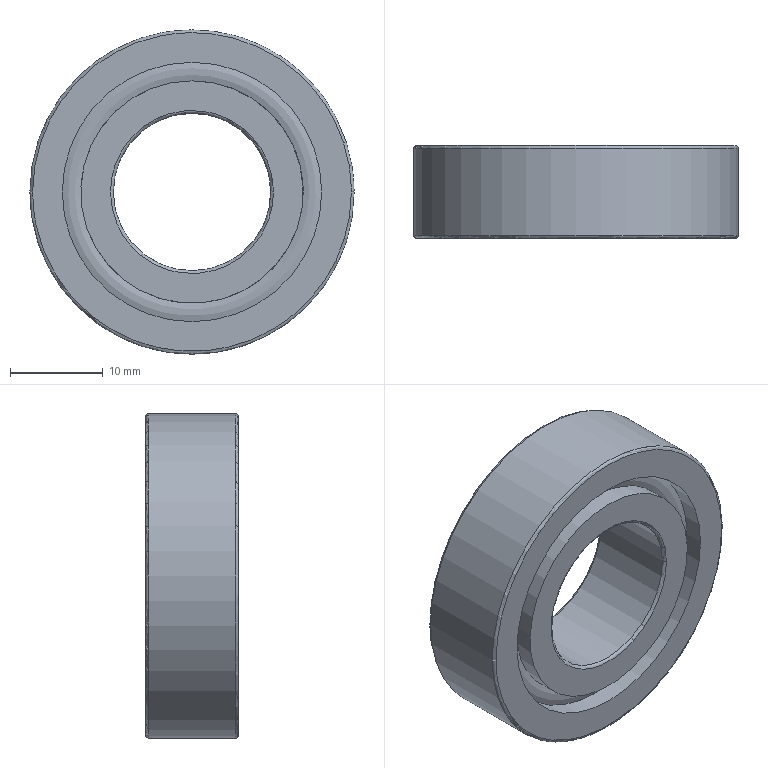Part | STEP file | 3 solids | 17 faces | box 35 x 10 x 35 mm | volume 6585 mm3 | torus 7 | cylinder 6 | plane 4 | commonest cylinder face diameters 24 x2 28 x2 17 x1 35 x1